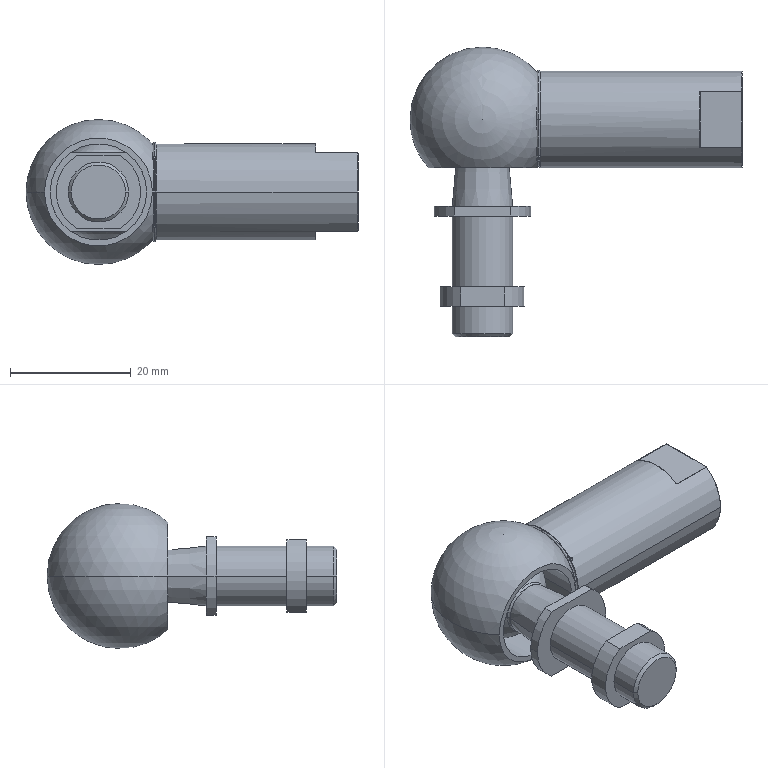Part | SolidWorks | features ICE 4, Fillet 2, Revolution 2, Chamfer 1, MirrorSolid 1, RevCut 1, Sweep 1 | 3 solids | 93 faces | box 55 x 48 x 24 mm | volume 13448 mm3 | cylinder 27 | torus 26 | plane 16 | sphere 14 | cone 6 | spline 4 | commonest cylinder face diameters 0.2 x8 16 x7 0.5 x4 10 x4 8.5 x2 14 x2